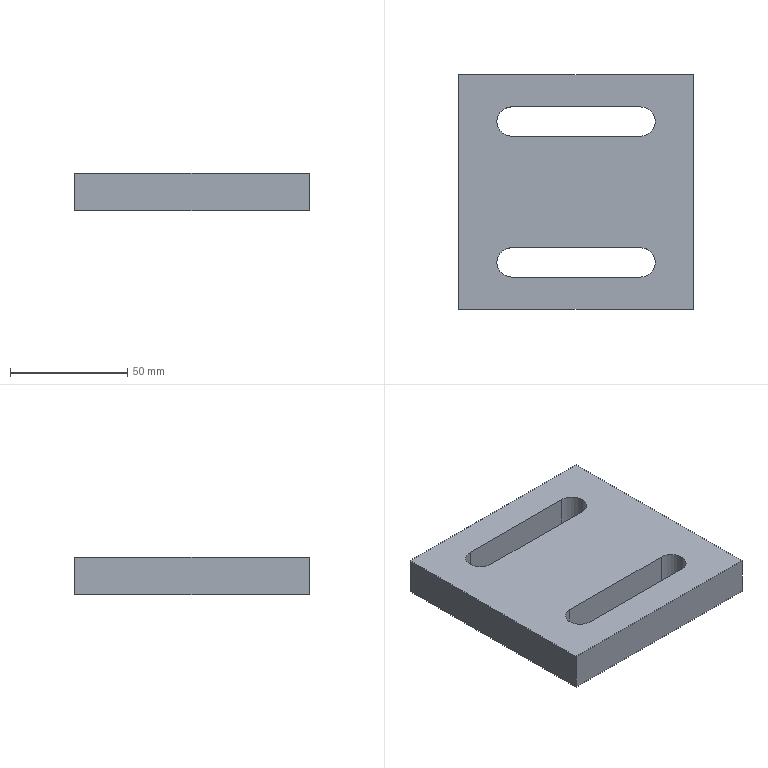Part | STEP file | 1 solid | 16 faces | box 100 x 100 x 16 mm | volume 134073 mm3 | plane 10 | cylinder 6 | commonest cylinder face diameters 12.5 x6
STEP:
#1=CARTESIAN_POINT('',(0.,0.,0.));
#2=DIRECTION('',(0.,0.,1.));
#3=DIRECTION('',(1.,0.,0.));
#4=AXIS2_PLACEMENT_3D('',#1,#2,#3);
#5=CARTESIAN_POINT('',(-27.5,36.25,16.));
#6=VERTEX_POINT('',#5);
#7=CARTESIAN_POINT('',(-27.5,36.25,0.));
#8=VERTEX_POINT('',#7);
#9=CARTESIAN_POINT('',(-27.5,36.25,16.));
#10=DIRECTION('',(0.,0.,-1.));
#11=VECTOR('',#10,1.);
#12=LINE('',#9,#11);
#13=CARTESIAN_POINT('',(-27.5,30.,16.));
#14=DIRECTION('',(0.,0.,-1.));
#15=DIRECTION('',(-1.,0.,0.));
#16=AXIS2_PLACEMENT_3D('',#13,#14,#15);
#17=CYLINDRICAL_SURFACE('',#16,6.25);
#18=CARTESIAN_POINT('',(1.571,0.));
#19=DIRECTION('',(0.,1.));
#20=VECTOR('',#19,1.);
#21=LINE('',#18,#20);
#22=(GEOMETRIC_REPRESENTATION_CONTEXT(2)PARAMETRIC_REPRESENTATION_CONTEXT()REPRESENTATION_CONTEXT('',''));
#23=DEFINITIONAL_REPRESENTATION('',(#21),#22);
#24=PCURVE('',#17,#23);
#25=CARTESIAN_POINT('',(-27.5,36.25,16.));
#26=DIRECTION('',(0.,-1.,0.));
#27=DIRECTION('',(0.,0.,-1.));
#28=AXIS2_PLACEMENT_3D('',#25,#26,#27);
#29=PLANE('',#28);
#30=CARTESIAN_POINT('',(0.,0.));
#31=DIRECTION('',(1.,0.));
#32=VECTOR('',#31,1.);
#33=LINE('',#30,#32);
#34=(GEOMETRIC_REPRESENTATION_CONTEXT(2)PARAMETRIC_REPRESENTATION_CONTEXT()REPRESENTATION_CONTEXT('',''));
#35=DEFINITIONAL_REPRESENTATION('',(#33),#34);
#36=PCURVE('',#29,#35);
#37=SURFACE_CURVE('',#12,(#24,#36),.PCURVE_S1.);
#38=EDGE_CURVE('',#6,#8,#37,.T.);
#39=ORIENTED_EDGE('',*,*,#38,.T.);
#40=CARTESIAN_POINT('',(-33.75,30.,0.));
#41=VERTEX_POINT('',#40);
#42=CARTESIAN_POINT('',(-27.5,30.,0.));
#43=DIRECTION('',(0.,0.,1.));
#44=DIRECTION('',(1.,0.,0.));
#45=AXIS2_PLACEMENT_3D('',#42,#43,#44);
#46=CIRCLE('',#45,6.25);
#47=CARTESIAN_POINT('',(3.142,16.));
#48=DIRECTION('',(-1.,0.));
#49=VECTOR('',#48,1.);
#50=LINE('',#47,#49);
#51=(GEOMETRIC_REPRESENTATION_CONTEXT(2)PARAMETRIC_REPRESENTATION_CONTEXT()REPRESENTATION_CONTEXT('',''));
#52=DEFINITIONAL_REPRESENTATION('',(#50),#51);
#53=PCURVE('',#17,#52);
#54=CARTESIAN_POINT('',(0.,0.,0.));
#55=DIRECTION('',(0.,0.,1.));
#56=DIRECTION('',(1.,0.,0.));
#57=AXIS2_PLACEMENT_3D('',#54,#55,#56);
#58=PLANE('',#57);
#59=CARTESIAN_POINT('',(-27.5,30.));
#60=DIRECTION('',(1.,0.));
#61=AXIS2_PLACEMENT_2D('',#59,#60);
#62=CIRCLE('',#61,6.25);
#63=(GEOMETRIC_REPRESENTATION_CONTEXT(2)PARAMETRIC_REPRESENTATION_CONTEXT()REPRESENTATION_CONTEXT('',''));
#64=DEFINITIONAL_REPRESENTATION('',(#62),#63);
#65=PCURVE('',#58,#64);
#66=SURFACE_CURVE('',#46,(#53,#65),.PCURVE_S1.);
#67=EDGE_CURVE('',#8,#41,#66,.T.);
#68=ORIENTED_EDGE('',*,*,#67,.T.);
#69=CARTESIAN_POINT('',(-33.75,30.,16.));
#70=VERTEX_POINT('',#69);
#71=CARTESIAN_POINT('',(-33.75,30.,16.));
#72=DIRECTION('',(0.,0.,-1.));
#73=VECTOR('',#72,1.);
#74=LINE('',#71,#73);
#75=CARTESIAN_POINT('',(0.,0.));
#76=DIRECTION('',(0.,1.));
#77=VECTOR('',#76,1.);
#78=LINE('',#75,#77);
#79=(GEOMETRIC_REPRESENTATION_CONTEXT(2)PARAMETRIC_REPRESENTATION_CONTEXT()REPRESENTATION_CONTEXT('',''));
#80=DEFINITIONAL_REPRESENTATION('',(#78),#79);
#81=PCURVE('',#17,#80);
#82=CARTESIAN_POINT('',(-27.5,30.,16.));
#83=DIRECTION('',(0.,0.,-1.));
#84=DIRECTION('',(-1.,0.,0.));
#85=AXIS2_PLACEMENT_3D('',#82,#83,#84);
#86=CYLINDRICAL_SURFACE('',#85,6.25);
#87=CARTESIAN_POINT('',(6.283,0.));
#88=DIRECTION('',(0.,1.));
#89=VECTOR('',#88,1.);
#90=LINE('',#87,#89);
#91=(GEOMETRIC_REPRESENTATION_CONTEXT(2)PARAMETRIC_REPRESENTATION_CONTEXT()REPRESENTATION_CONTEXT('',''));
#92=DEFINITIONAL_REPRESENTATION('',(#90),#91);
#93=PCURVE('',#86,#92);
#94=SURFACE_CURVE('',#74,(#81,#93),.PCURVE_S1.);
#95=EDGE_CURVE('',#70,#41,#94,.T.);
#96=ORIENTED_EDGE('',*,*,#95,.F.);
#97=CARTESIAN_POINT('',(-27.5,30.,16.));
#98=DIRECTION('',(0.,0.,1.));
#99=DIRECTION('',(1.,0.,0.));
#100=AXIS2_PLACEMENT_3D('',#97,#98,#99);
#101=CIRCLE('',#100,6.25);
#102=CARTESIAN_POINT('',(3.142,0.));
#103=DIRECTION('',(-1.,0.));
#104=VECTOR('',#103,1.);
#105=LINE('',#102,#104);
#106=(GEOMETRIC_REPRESENTATION_CONTEXT(2)PARAMETRIC_REPRESENTATION_CONTEXT()REPRESENTATION_CONTEXT('',''));
#107=DEFINITIONAL_REPRESENTATION('',(#105),#106);
#108=PCURVE('',#17,#107);
#109=CARTESIAN_POINT('',(0.,0.,16.));
#110=DIRECTION('',(0.,0.,1.));
#111=DIRECTION('',(1.,0.,0.));
#112=AXIS2_PLACEMENT_3D('',#109,#110,#111);
#113=PLANE('',#112);
#114=CARTESIAN_POINT('',(-27.5,30.));
#115=DIRECTION('',(1.,0.));
#116=AXIS2_PLACEMENT_2D('',#114,#115);
#117=CIRCLE('',#116,6.25);
#118=(GEOMETRIC_REPRESENTATION_CONTEXT(2)PARAMETRIC_REPRESENTATION_CONTEXT()REPRESENTATION_CONTEXT('',''));
#119=DEFINITIONAL_REPRESENTATION('',(#117),#118);
#120=PCURVE('',#113,#119);
#121=SURFACE_CURVE('',#101,(#108,#120),.PCURVE_S1.);
#122=EDGE_CURVE('',#6,#70,#121,.T.);
#123=ORIENTED_EDGE('',*,*,#122,.F.);
#124=EDGE_LOOP('',(#39,#68,#96,#123));
#125=FACE_BOUND('',#124,.F.);
#126=ADVANCED_FACE('',(#125),#17,.F.);
#127=CARTESIAN_POINT('',(-27.5,-23.75,16.));
#128=VERTEX_POINT('',#127);
#129=CARTESIAN_POINT('',(-27.5,-23.75,0.));
#130=VERTEX_POINT('',#129);
#131=CARTESIAN_POINT('',(-27.5,-23.75,16.));
#132=DIRECTION('',(0.,0.,-1.));
#133=VECTOR('',#132,1.);
#134=LINE('',#131,#133);
#135=CARTESIAN_POINT('',(-27.5,-30.,16.));
#136=DIRECTION('',(0.,0.,-1.));
#137=DIRECTION('',(-1.,0.,0.));
#138=AXIS2_PLACEMENT_3D('',#135,#136,#137);
#139=CYLINDRICAL_SURFACE('',#138,6.25);
#140=CARTESIAN_POINT('',(1.571,0.));
#141=DIRECTION('',(0.,1.));
#142=VECTOR('',#141,1.);
#143=LINE('',#140,#142);
#144=(GEOMETRIC_REPRESENTATION_CONTEXT(2)PARAMETRIC_REPRESENTATION_CONTEXT()REPRESENTATION_CONTEXT('',''));
#145=DEFINITIONAL_REPRESENTATION('',(#143),#144);
#146=PCURVE('',#139,#145);
#147=CARTESIAN_POINT('',(-27.5,-23.75,16.));
#148=DIRECTION('',(0.,-1.,0.));
#149=DIRECTION('',(1.,0.,0.));
#150=AXIS2_PLACEMENT_3D('',#147,#148,#149);
#151=PLANE('',#150);
#152=CARTESIAN_POINT('',(0.,0.));
#153=DIRECTION('',(0.,-1.));
#154=VECTOR('',#153,1.);
#155=LINE('',#152,#154);
#156=(GEOMETRIC_REPRESENTATION_CONTEXT(2)PARAMETRIC_REPRESENTATION_CONTEXT()REPRESENTATION_CONTEXT('',''));
#157=DEFINITIONAL_REPRESENTATION('',(#155),#156);
#158=PCURVE('',#151,#157);
#159=SURFACE_CURVE('',#134,(#146,#158),.PCURVE_S1.);
#160=EDGE_CURVE('',#128,#130,#159,.T.);
#161=ORIENTED_EDGE('',*,*,#160,.T.);
#162=CARTESIAN_POINT('',(-33.75,-30.,0.));
#163=VERTEX_POINT('',#162);
#164=CARTESIAN_POINT('',(-27.5,-30.,0.));
#165=DIRECTION('',(0.,0.,1.));
#166=DIRECTION('',(1.,0.,0.));
#167=AXIS2_PLACEMENT_3D('',#164,#165,#166);
#168=CIRCLE('',#167,6.25);
#169=CARTESIAN_POINT('',(3.142,16.));
#170=DIRECTION('',(-1.,0.));
#171=VECTOR('',#170,1.);
#172=LINE('',#169,#171);
#173=(GEOMETRIC_REPRESENTATION_CONTEXT(2)PARAMETRIC_REPRESENTATION_CONTEXT()REPRESENTATION_CONTEXT('',''));
#174=DEFINITIONAL_REPRESENTATION('',(#172),#173);
#175=PCURVE('',#139,#174);
#176=CARTESIAN_POINT('',(-27.5,-30.));
#177=DIRECTION('',(1.,0.));
#178=AXIS2_PLACEMENT_2D('',#176,#177);
#179=CIRCLE('',#178,6.25);
#180=(GEOMETRIC_REPRESENTATION_CONTEXT(2)PARAMETRIC_REPRESENTATION_CONTEXT()REPRESENTATION_CONTEXT('',''));
#181=DEFINITIONAL_REPRESENTATION('',(#179),#180);
#182=PCURVE('',#58,#181);
#183=SURFACE_CURVE('',#168,(#175,#182),.PCURVE_S1.);
#184=EDGE_CURVE('',#130,#163,#183,.T.);
#185=ORIENTED_EDGE('',*,*,#184,.T.);
#186=CARTESIAN_POINT('',(-33.75,-30.,16.));
#187=VERTEX_POINT('',#186);
#188=CARTESIAN_POINT('',(-33.75,-30.,16.));
#189=DIRECTION('',(0.,0.,-1.));
#190=VECTOR('',#189,1.);
#191=LINE('',#188,#190);
#192=CARTESIAN_POINT('',(0.,0.));
#193=DIRECTION('',(0.,1.));
#194=VECTOR('',#193,1.);
#195=LINE('',#192,#194);
#196=(GEOMETRIC_REPRESENTATION_CONTEXT(2)PARAMETRIC_REPRESENTATION_CONTEXT()REPRESENTATION_CONTEXT('',''));
#197=DEFINITIONAL_REPRESENTATION('',(#195),#196);
#198=PCURVE('',#139,#197);
#199=CARTESIAN_POINT('',(-27.5,-30.,16.));
#200=DIRECTION('',(0.,0.,-1.));
#201=DIRECTION('',(-1.,0.,0.));
#202=AXIS2_PLACEMENT_3D('',#199,#200,#201);
#203=CYLINDRICAL_SURFACE('',#202,6.25);
#204=CARTESIAN_POINT('',(6.283,0.));
#205=DIRECTION('',(0.,1.));
#206=VECTOR('',#205,1.);
#207=LINE('',#204,#206);
#208=(GEOMETRIC_REPRESENTATION_CONTEXT(2)PARAMETRIC_REPRESENTATION_CONTEXT()REPRESENTATION_CONTEXT('',''));
#209=DEFINITIONAL_REPRESENTATION('',(#207),#208);
#210=PCURVE('',#203,#209);
#211=SURFACE_CURVE('',#191,(#198,#210),.PCURVE_S1.);
#212=EDGE_CURVE('',#187,#163,#211,.T.);
#213=ORIENTED_EDGE('',*,*,#212,.F.);
#214=CARTESIAN_POINT('',(-27.5,-30.,16.));
#215=DIRECTION('',(0.,0.,1.));
#216=DIRECTION('',(1.,0.,0.));
#217=AXIS2_PLACEMENT_3D('',#214,#215,#216);
#218=CIRCLE('',#217,6.25);
#219=CARTESIAN_POINT('',(3.142,0.));
#220=DIRECTION('',(-1.,0.));
#221=VECTOR('',#220,1.);
#222=LINE('',#219,#221);
#223=(GEOMETRIC_REPRESENTATION_CONTEXT(2)PARAMETRIC_REPRESENTATION_CONTEXT()REPRESENTATION_CONTEXT('',''));
#224=DEFINITIONAL_REPRESENTATION('',(#222),#223);
#225=PCURVE('',#139,#224);
#226=CARTESIAN_POINT('',(-27.5,-30.));
#227=DIRECTION('',(1.,0.));
#228=AXIS2_PLACEMENT_2D('',#226,#227);
#229=CIRCLE('',#228,6.25);
#230=(GEOMETRIC_REPRESENTATION_CONTEXT(2)PARAMETRIC_REPRESENTATION_CONTEXT()REPRESENTATION_CONTEXT('',''));
#231=DEFINITIONAL_REPRESENTATION('',(#229),#230);
#232=PCURVE('',#113,#231);
#233=SURFACE_CURVE('',#218,(#225,#232),.PCURVE_S1.);
#234=EDGE_CURVE('',#128,#187,#233,.T.);
#235=ORIENTED_EDGE('',*,*,#234,.F.);
#236=EDGE_LOOP('',(#161,#185,#213,#235));
#237=FACE_BOUND('',#236,.F.);
#238=ADVANCED_FACE('',(#237),#139,.F.);
#239=CARTESIAN_POINT('',(50.,-50.,16.));
#240=VERTEX_POINT('',#239);
#241=CARTESIAN_POINT('',(50.,50.,16.));
#242=VERTEX_POINT('',#241);
#243=CARTESIAN_POINT('',(50.,-10.,16.));
#244=DIRECTION('',(0.,1.,0.));
#245=VECTOR('',#244,1.);
#246=LINE('',#243,#245);
#247=CARTESIAN_POINT('',(50.,-10.));
#248=DIRECTION('',(0.,1.));
#249=VECTOR('',#248,1.);
#250=LINE('',#247,#249);
#251=(GEOMETRIC_REPRESENTATION_CONTEXT(2)PARAMETRIC_REPRESENTATION_CONTEXT()REPRESENTATION_CONTEXT('',''));
#252=DEFINITIONAL_REPRESENTATION('',(#250),#251);
#253=PCURVE('',#113,#252);
#254=CARTESIAN_POINT('',(50.,50.,16.));
#255=DIRECTION('',(-1.,0.,0.));
#256=DIRECTION('',(0.,-1.,0.));
#257=AXIS2_PLACEMENT_3D('',#254,#255,#256);
#258=PLANE('',#257);
#259=CARTESIAN_POINT('',(60.,0.));
#260=DIRECTION('',(-1.,0.));
#261=VECTOR('',#260,1.);
#262=LINE('',#259,#261);
#263=(GEOMETRIC_REPRESENTATION_CONTEXT(2)PARAMETRIC_REPRESENTATION_CONTEXT()REPRESENTATION_CONTEXT('',''));
#264=DEFINITIONAL_REPRESENTATION('',(#262),#263);
#265=PCURVE('',#258,#264);
#266=SURFACE_CURVE('',#246,(#253,#265),.PCURVE_S1.);
#267=EDGE_CURVE('',#240,#242,#266,.T.);
#268=ORIENTED_EDGE('',*,*,#267,.T.);
#269=CARTESIAN_POINT('',(-50.,50.,16.));
#270=VERTEX_POINT('',#269);
#271=CARTESIAN_POINT('',(-50.,50.,16.));
#272=DIRECTION('',(-1.,0.,0.));
#273=VECTOR('',#272,1.);
#274=LINE('',#271,#273);
#275=CARTESIAN_POINT('',(-50.,50.));
#276=DIRECTION('',(-1.,0.));
#277=VECTOR('',#276,1.);
#278=LINE('',#275,#277);
#279=(GEOMETRIC_REPRESENTATION_CONTEXT(2)PARAMETRIC_REPRESENTATION_CONTEXT()REPRESENTATION_CONTEXT('',''));
#280=DEFINITIONAL_REPRESENTATION('',(#278),#279);
#281=PCURVE('',#113,#280);
#282=CARTESIAN_POINT('',(-50.,50.,16.));
#283=DIRECTION('',(0.,-1.,0.));
#284=DIRECTION('',(0.,0.,-1.));
#285=AXIS2_PLACEMENT_3D('',#282,#283,#284);
#286=PLANE('',#285);
#287=CARTESIAN_POINT('',(0.,0.));
#288=DIRECTION('',(0.,-1.));
#289=VECTOR('',#288,1.);
#290=LINE('',#287,#289);
#291=(GEOMETRIC_REPRESENTATION_CONTEXT(2)PARAMETRIC_REPRESENTATION_CONTEXT()REPRESENTATION_CONTEXT('',''));
#292=DEFINITIONAL_REPRESENTATION('',(#290),#291);
#293=PCURVE('',#286,#292);
#294=SURFACE_CURVE('',#274,(#281,#293),.PCURVE_S1.);
#295=EDGE_CURVE('',#242,#270,#294,.T.);
#296=ORIENTED_EDGE('',*,*,#295,.T.);
#297=CARTESIAN_POINT('',(-50.,-50.,16.));
#298=VERTEX_POINT('',#297);
#299=CARTESIAN_POINT('',(-50.,50.,16.));
#300=DIRECTION('',(0.,-1.,0.));
#301=VECTOR('',#300,1.);
#302=LINE('',#299,#301);
#303=CARTESIAN_POINT('',(-50.,50.));
#304=DIRECTION('',(0.,-1.));
#305=VECTOR('',#304,1.);
#306=LINE('',#303,#305);
#307=(GEOMETRIC_REPRESENTATION_CONTEXT(2)PARAMETRIC_REPRESENTATION_CONTEXT()REPRESENTATION_CONTEXT('',''));
#308=DEFINITIONAL_REPRESENTATION('',(#306),#307);
#309=PCURVE('',#113,#308);
#310=CARTESIAN_POINT('',(-50.,50.,16.));
#311=DIRECTION('',(1.,0.,0.));
#312=DIRECTION('',(0.,1.,0.));
#313=AXIS2_PLACEMENT_3D('',#310,#311,#312);
#314=PLANE('',#313);
#315=CARTESIAN_POINT('',(0.,0.));
#316=DIRECTION('',(-1.,0.));
#317=VECTOR('',#316,1.);
#318=LINE('',#315,#317);
#319=(GEOMETRIC_REPRESENTATION_CONTEXT(2)PARAMETRIC_REPRESENTATION_CONTEXT()REPRESENTATION_CONTEXT('',''));
#320=DEFINITIONAL_REPRESENTATION('',(#318),#319);
#321=PCURVE('',#314,#320);
#322=SURFACE_CURVE('',#302,(#309,#321),.PCURVE_S1.);
#323=EDGE_CURVE('',#270,#298,#322,.T.);
#324=ORIENTED_EDGE('',*,*,#323,.T.);
#325=CARTESIAN_POINT('',(-50.,-50.,16.));
#326=DIRECTION('',(1.,0.,0.));
#327=VECTOR('',#326,1.);
#328=LINE('',#325,#327);
#329=CARTESIAN_POINT('',(-50.,-50.));
#330=DIRECTION('',(1.,0.));
#331=VECTOR('',#330,1.);
#332=LINE('',#329,#331);
#333=(GEOMETRIC_REPRESENTATION_CONTEXT(2)PARAMETRIC_REPRESENTATION_CONTEXT()REPRESENTATION_CONTEXT('',''));
#334=DEFINITIONAL_REPRESENTATION('',(#332),#333);
#335=PCURVE('',#113,#334);
#336=CARTESIAN_POINT('',(-50.,-50.,16.));
#337=DIRECTION('',(0.,1.,0.));
#338=DIRECTION('',(0.,0.,1.));
#339=AXIS2_PLACEMENT_3D('',#336,#337,#338);
#340=PLANE('',#339);
#341=CARTESIAN_POINT('',(0.,0.));
#342=DIRECTION('',(0.,1.));
#343=VECTOR('',#342,1.);
#344=LINE('',#341,#343);
#345=(GEOMETRIC_REPRESENTATION_CONTEXT(2)PARAMETRIC_REPRESENTATION_CONTEXT()REPRESENTATION_CONTEXT('',''));
#346=DEFINITIONAL_REPRESENTATION('',(#344),#345);
#347=PCURVE('',#340,#346);
#348=SURFACE_CURVE('',#328,(#335,#347),.PCURVE_S1.);
#349=EDGE_CURVE('',#298,#240,#348,.T.);
#350=ORIENTED_EDGE('',*,*,#349,.T.);
#351=EDGE_LOOP('',(#268,#296,#324,#350));
#352=FACE_BOUND('',#351,.T.);
#353=CARTESIAN_POINT('',(-27.5,-36.25,16.));
#354=VERTEX_POINT('',#353);
#355=CARTESIAN_POINT('',(27.5,-36.25,16.));
#356=VERTEX_POINT('',#355);
#357=CARTESIAN_POINT('',(-27.5,-36.25,16.));
#358=DIRECTION('',(1.,0.,0.));
#359=VECTOR('',#358,1.);
#360=LINE('',#357,#359);
#361=CARTESIAN_POINT('',(-27.5,-36.25));
#362=DIRECTION('',(1.,0.));
#363=VECTOR('',#362,1.);
#364=LINE('',#361,#363);
#365=(GEOMETRIC_REPRESENTATION_CONTEXT(2)PARAMETRIC_REPRESENTATION_CONTEXT()REPRESENTATION_CONTEXT('',''));
#366=DEFINITIONAL_REPRESENTATION('',(#364),#365);
#367=PCURVE('',#113,#366);
#368=CARTESIAN_POINT('',(-27.5,-36.25,16.));
#369=DIRECTION('',(0.,1.,0.));
#370=DIRECTION('',(0.,0.,1.));
#371=AXIS2_PLACEMENT_3D('',#368,#369,#370);
#372=PLANE('',#371);
#373=CARTESIAN_POINT('',(0.,0.));
#374=DIRECTION('',(0.,1.));
#375=VECTOR('',#374,1.);
#376=LINE('',#373,#375);
#377=(GEOMETRIC_REPRESENTATION_CONTEXT(2)PARAMETRIC_REPRESENTATION_CONTEXT()REPRESENTATION_CONTEXT('',''));
#378=DEFINITIONAL_REPRESENTATION('',(#376),#377);
#379=PCURVE('',#372,#378);
#380=SURFACE_CURVE('',#360,(#367,#379),.PCURVE_S1.);
#381=EDGE_CURVE('',#354,#356,#380,.T.);
#382=ORIENTED_EDGE('',*,*,#381,.F.);
#383=CARTESIAN_POINT('',(-27.5,-30.,16.));
#384=DIRECTION('',(0.,0.,1.));
#385=DIRECTION('',(1.,0.,0.));
#386=AXIS2_PLACEMENT_3D('',#383,#384,#385);
#387=CIRCLE('',#386,6.25);
#388=CARTESIAN_POINT('',(-27.5,-30.));
#389=DIRECTION('',(1.,0.));
#390=AXIS2_PLACEMENT_2D('',#388,#389);
#391=CIRCLE('',#390,6.25);
#392=(GEOMETRIC_REPRESENTATION_CONTEXT(2)PARAMETRIC_REPRESENTATION_CONTEXT()REPRESENTATION_CONTEXT('',''));
#393=DEFINITIONAL_REPRESENTATION('',(#391),#392);
#394=PCURVE('',#113,#393);
#395=CARTESIAN_POINT('',(9.425,0.));
#396=DIRECTION('',(-1.,0.));
#397=VECTOR('',#396,1.);
#398=LINE('',#395,#397);
#399=(GEOMETRIC_REPRESENTATION_CONTEXT(2)PARAMETRIC_REPRESENTATION_CONTEXT()REPRESENTATION_CONTEXT('',''));
#400=DEFINITIONAL_REPRESENTATION('',(#398),#399);
#401=PCURVE('',#203,#400);
#402=SURFACE_CURVE('',#387,(#394,#401),.PCURVE_S1.);
#403=EDGE_CURVE('',#187,#354,#402,.T.);
#404=ORIENTED_EDGE('',*,*,#403,.F.);
#405=ORIENTED_EDGE('',*,*,#234,.F.);
#406=CARTESIAN_POINT('',(27.5,-23.75,16.));
#407=VERTEX_POINT('',#406);
#408=CARTESIAN_POINT('',(-27.5,-23.75,16.));
#409=DIRECTION('',(-1.,0.,0.));
#410=VECTOR('',#409,1.);
#411=LINE('',#408,#410);
#412=CARTESIAN_POINT('',(-27.5,-23.75));
#413=DIRECTION('',(-1.,0.));
#414=VECTOR('',#413,1.);
#415=LINE('',#412,#414);
#416=(GEOMETRIC_REPRESENTATION_CONTEXT(2)PARAMETRIC_REPRESENTATION_CONTEXT()REPRESENTATION_CONTEXT('',''));
#417=DEFINITIONAL_REPRESENTATION('',(#415),#416);
#418=PCURVE('',#113,#417);
#419=CARTESIAN_POINT('',(0.,0.));
#420=DIRECTION('',(-1.,0.));
#421=VECTOR('',#420,1.);
#422=LINE('',#419,#421);
#423=(GEOMETRIC_REPRESENTATION_CONTEXT(2)PARAMETRIC_REPRESENTATION_CONTEXT()REPRESENTATION_CONTEXT('',''));
#424=DEFINITIONAL_REPRESENTATION('',(#422),#423);
#425=PCURVE('',#151,#424);
#426=SURFACE_CURVE('',#411,(#418,#425),.PCURVE_S1.);
#427=EDGE_CURVE('',#407,#128,#426,.T.);
#428=ORIENTED_EDGE('',*,*,#427,.F.);
#429=CARTESIAN_POINT('',(27.5,-30.,16.));
#430=DIRECTION('',(0.,0.,1.));
#431=DIRECTION('',(1.,0.,0.));
#432=AXIS2_PLACEMENT_3D('',#429,#430,#431);
#433=CIRCLE('',#432,6.25);
#434=CARTESIAN_POINT('',(27.5,-30.));
#435=DIRECTION('',(1.,0.));
#436=AXIS2_PLACEMENT_2D('',#434,#435);
#437=CIRCLE('',#436,6.25);
#438=(GEOMETRIC_REPRESENTATION_CONTEXT(2)PARAMETRIC_REPRESENTATION_CONTEXT()REPRESENTATION_CONTEXT('',''));
#439=DEFINITIONAL_REPRESENTATION('',(#437),#438);
#440=PCURVE('',#113,#439);
#441=CARTESIAN_POINT('',(27.5,-30.,16.));
#442=DIRECTION('',(0.,0.,-1.));
#443=DIRECTION('',(-1.,0.,0.));
#444=AXIS2_PLACEMENT_3D('',#441,#442,#443);
#445=CYLINDRICAL_SURFACE('',#444,6.25);
#446=CARTESIAN_POINT('',(9.425,0.));
#447=DIRECTION('',(-1.,0.));
#448=VECTOR('',#447,1.);
#449=LINE('',#446,#448);
#450=(GEOMETRIC_REPRESENTATION_CONTEXT(2)PARAMETRIC_REPRESENTATION_CONTEXT()REPRESENTATION_CONTEXT('',''));
#451=DEFINITIONAL_REPRESENTATION('',(#449),#450);
#452=PCURVE('',#445,#451);
#453=SURFACE_CURVE('',#433,(#440,#452),.PCURVE_S1.);
#454=EDGE_CURVE('',#356,#407,#453,.T.);
#455=ORIENTED_EDGE('',*,*,#454,.F.);
#456=EDGE_LOOP('',(#382,#404,#405,#428,#455));
#457=FACE_BOUND('',#456,.T.);
#458=CARTESIAN_POINT('',(-27.5,23.75,16.));
#459=VERTEX_POINT('',#458);
#460=CARTESIAN_POINT('',(27.5,23.75,16.));
#461=VERTEX_POINT('',#460);
#462=CARTESIAN_POINT('',(-27.5,23.75,16.));
#463=DIRECTION('',(1.,0.,0.));
#464=VECTOR('',#463,1.);
#465=LINE('',#462,#464);
#466=CARTESIAN_POINT('',(-27.5,23.75));
#467=DIRECTION('',(1.,0.));
#468=VECTOR('',#467,1.);
#469=LINE('',#466,#468);
#470=(GEOMETRIC_REPRESENTATION_CONTEXT(2)PARAMETRIC_REPRESENTATION_CONTEXT()REPRESENTATION_CONTEXT('',''));
#471=DEFINITIONAL_REPRESENTATION('',(#469),#470);
#472=PCURVE('',#113,#471);
#473=CARTESIAN_POINT('',(-27.5,23.75,16.));
#474=DIRECTION('',(0.,1.,0.));
#475=DIRECTION('',(0.,0.,1.));
#476=AXIS2_PLACEMENT_3D('',#473,#474,#475);
#477=PLANE('',#476);
#478=CARTESIAN_POINT('',(0.,0.));
#479=DIRECTION('',(0.,1.));
#480=VECTOR('',#479,1.);
#481=LINE('',#478,#480);
#482=(GEOMETRIC_REPRESENTATION_CONTEXT(2)PARAMETRIC_REPRESENTATION_CONTEXT()REPRESENTATION_CONTEXT('',''));
#483=DEFINITIONAL_REPRESENTATION('',(#481),#482);
#484=PCURVE('',#477,#483);
#485=SURFACE_CURVE('',#465,(#472,#484),.PCURVE_S1.);
#486=EDGE_CURVE('',#459,#461,#485,.T.);
#487=ORIENTED_EDGE('',*,*,#486,.F.);
#488=CARTESIAN_POINT('',(-27.5,30.,16.));
#489=DIRECTION('',(0.,0.,1.));
#490=DIRECTION('',(1.,0.,0.));
#491=AXIS2_PLACEMENT_3D('',#488,#489,#490);
#492=CIRCLE('',#491,6.25);
#493=CARTESIAN_POINT('',(-27.5,30.));
#494=DIRECTION('',(1.,0.));
#495=AXIS2_PLACEMENT_2D('',#493,#494);
#496=CIRCLE('',#495,6.25);
#497=(GEOMETRIC_REPRESENTATION_CONTEXT(2)PARAMETRIC_REPRESENTATION_CONTEXT()REPRESENTATION_CONTEXT('',''));
#498=DEFINITIONAL_REPRESENTATION('',(#496),#497);
#499=PCURVE('',#113,#498);
#500=CARTESIAN_POINT('',(9.425,0.));
#501=DIRECTION('',(-1.,0.));
#502=VECTOR('',#501,1.);
#503=LINE('',#500,#502);
#504=(GEOMETRIC_REPRESENTATION_CONTEXT(2)PARAMETRIC_REPRESENTATION_CONTEXT()REPRESENTATION_CONTEXT('',''));
#505=DEFINITIONAL_REPRESENTATION('',(#503),#504);
#506=PCURVE('',#86,#505);
#507=SURFACE_CURVE('',#492,(#499,#506),.PCURVE_S1.);
#508=EDGE_CURVE('',#70,#459,#507,.T.);
#509=ORIENTED_EDGE('',*,*,#508,.F.);
#510=ORIENTED_EDGE('',*,*,#122,.F.);
#511=CARTESIAN_POINT('',(27.5,36.25,16.));
#512=VERTEX_POINT('',#511);
#513=CARTESIAN_POINT('',(-27.5,36.25,16.));
#514=DIRECTION('',(-1.,0.,0.));
#515=VECTOR('',#514,1.);
#516=LINE('',#513,#515);
#517=CARTESIAN_POINT('',(-27.5,36.25));
#518=DIRECTION('',(-1.,0.));
#519=VECTOR('',#518,1.);
#520=LINE('',#517,#519);
#521=(GEOMETRIC_REPRESENTATION_CONTEXT(2)PARAMETRIC_REPRESENTATION_CONTEXT()REPRESENTATION_CONTEXT('',''));
#522=DEFINITIONAL_REPRESENTATION('',(#520),#521);
#523=PCURVE('',#113,#522);
#524=CARTESIAN_POINT('',(0.,0.));
#525=DIRECTION('',(0.,-1.));
#526=VECTOR('',#525,1.);
#527=LINE('',#524,#526);
#528=(GEOMETRIC_REPRESENTATION_CONTEXT(2)PARAMETRIC_REPRESENTATION_CONTEXT()REPRESENTATION_CONTEXT('',''));
#529=DEFINITIONAL_REPRESENTATION('',(#527),#528);
#530=PCURVE('',#29,#529);
#531=SURFACE_CURVE('',#516,(#523,#530),.PCURVE_S1.);
#532=EDGE_CURVE('',#512,#6,#531,.T.);
#533=ORIENTED_EDGE('',*,*,#532,.F.);
#534=CARTESIAN_POINT('',(27.5,30.,16.));
#535=DIRECTION('',(0.,0.,1.));
#536=DIRECTION('',(1.,0.,0.));
#537=AXIS2_PLACEMENT_3D('',#534,#535,#536);
#538=CIRCLE('',#537,6.25);
#539=CARTESIAN_POINT('',(27.5,30.));
#540=DIRECTION('',(1.,0.));
#541=AXIS2_PLACEMENT_2D('',#539,#540);
#542=CIRCLE('',#541,6.25);
#543=(GEOMETRIC_REPRESENTATION_CONTEXT(2)PARAMETRIC_REPRESENTATION_CONTEXT()REPRESENTATION_CONTEXT('',''));
#544=DEFINITIONAL_REPRESENTATION('',(#542),#543);
#545=PCURVE('',#113,#544);
#546=CARTESIAN_POINT('',(27.5,30.,16.));
#547=DIRECTION('',(0.,0.,-1.));
#548=DIRECTION('',(-1.,0.,0.));
#549=AXIS2_PLACEMENT_3D('',#546,#547,#548);
#550=CYLINDRICAL_SURFACE('',#549,6.25);
#551=CARTESIAN_POINT('',(9.425,0.));
#552=DIRECTION('',(-1.,0.));
#553=VECTOR('',#552,1.);
#554=LINE('',#551,#553);
#555=(GEOMETRIC_REPRESENTATION_CONTEXT(2)PARAMETRIC_REPRESENTATION_CONTEXT()REPRESENTATION_CONTEXT('',''));
#556=DEFINITIONAL_REPRESENTATION('',(#554),#555);
#557=PCURVE('',#550,#556);
#558=SURFACE_CURVE('',#538,(#545,#557),.PCURVE_S1.);
#559=EDGE_CURVE('',#461,#512,#558,.T.);
#560=ORIENTED_EDGE('',*,*,#559,.F.);
#561=EDGE_LOOP('',(#487,#509,#510,#533,#560));
#562=FACE_BOUND('',#561,.T.);
#563=ADVANCED_FACE('',(#352,#457,#562),#113,.T.);
#564=ORIENTED_EDGE('',*,*,#184,.T.);
#565=CARTESIAN_POINT('',(-27.5,-36.25,0.));
#566=VERTEX_POINT('',#565);
#567=CARTESIAN_POINT('',(-27.5,-30.,0.));
#568=DIRECTION('',(0.,0.,1.));
#569=DIRECTION('',(1.,0.,0.));
#570=AXIS2_PLACEMENT_3D('',#567,#568,#569);
#571=CIRCLE('',#570,6.25);
#572=CARTESIAN_POINT('',(-27.5,-30.));
#573=DIRECTION('',(1.,0.));
#574=AXIS2_PLACEMENT_2D('',#572,#573);
#575=CIRCLE('',#574,6.25);
#576=(GEOMETRIC_REPRESENTATION_CONTEXT(2)PARAMETRIC_REPRESENTATION_CONTEXT()REPRESENTATION_CONTEXT('',''));
#577=DEFINITIONAL_REPRESENTATION('',(#575),#576);
#578=PCURVE('',#58,#577);
#579=CARTESIAN_POINT('',(9.425,16.));
#580=DIRECTION('',(-1.,0.));
#581=VECTOR('',#580,1.);
#582=LINE('',#579,#581);
#583=(GEOMETRIC_REPRESENTATION_CONTEXT(2)PARAMETRIC_REPRESENTATION_CONTEXT()REPRESENTATION_CONTEXT('',''));
#584=DEFINITIONAL_REPRESENTATION('',(#582),#583);
#585=PCURVE('',#203,#584);
#586=SURFACE_CURVE('',#571,(#578,#585),.PCURVE_S1.);
#587=EDGE_CURVE('',#163,#566,#586,.T.);
#588=ORIENTED_EDGE('',*,*,#587,.T.);
#589=CARTESIAN_POINT('',(27.5,-36.25,0.));
#590=VERTEX_POINT('',#589);
#591=CARTESIAN_POINT('',(-27.5,-36.25,0.));
#592=DIRECTION('',(1.,0.,0.));
#593=VECTOR('',#592,1.);
#594=LINE('',#591,#593);
#595=CARTESIAN_POINT('',(-27.5,-36.25));
#596=DIRECTION('',(1.,0.));
#597=VECTOR('',#596,1.);
#598=LINE('',#595,#597);
#599=(GEOMETRIC_REPRESENTATION_CONTEXT(2)PARAMETRIC_REPRESENTATION_CONTEXT()REPRESENTATION_CONTEXT('',''));
#600=DEFINITIONAL_REPRESENTATION('',(#598),#599);
#601=PCURVE('',#58,#600);
#602=CARTESIAN_POINT('',(-16.,0.));
#603=DIRECTION('',(0.,1.));
#604=VECTOR('',#603,1.);
#605=LINE('',#602,#604);
#606=(GEOMETRIC_REPRESENTATION_CONTEXT(2)PARAMETRIC_REPRESENTATION_CONTEXT()REPRESENTATION_CONTEXT('',''));
#607=DEFINITIONAL_REPRESENTATION('',(#605),#606);
#608=PCURVE('',#372,#607);
#609=SURFACE_CURVE('',#594,(#601,#608),.PCURVE_S1.);
#610=EDGE_CURVE('',#566,#590,#609,.T.);
#611=ORIENTED_EDGE('',*,*,#610,.T.);
#612=CARTESIAN_POINT('',(27.5,-23.75,0.));
#613=VERTEX_POINT('',#612);
#614=CARTESIAN_POINT('',(27.5,-30.,0.));
#615=DIRECTION('',(0.,0.,1.));
#616=DIRECTION('',(1.,0.,0.));
#617=AXIS2_PLACEMENT_3D('',#614,#615,#616);
#618=CIRCLE('',#617,6.25);
#619=CARTESIAN_POINT('',(27.5,-30.));
#620=DIRECTION('',(1.,0.));
#621=AXIS2_PLACEMENT_2D('',#619,#620);
#622=CIRCLE('',#621,6.25);
#623=(GEOMETRIC_REPRESENTATION_CONTEXT(2)PARAMETRIC_REPRESENTATION_CONTEXT()REPRESENTATION_CONTEXT('',''));
#624=DEFINITIONAL_REPRESENTATION('',(#622),#623);
#625=PCURVE('',#58,#624);
#626=CARTESIAN_POINT('',(9.425,16.));
#627=DIRECTION('',(-1.,0.));
#628=VECTOR('',#627,1.);
#629=LINE('',#626,#628);
#630=(GEOMETRIC_REPRESENTATION_CONTEXT(2)PARAMETRIC_REPRESENTATION_CONTEXT()REPRESENTATION_CONTEXT('',''));
#631=DEFINITIONAL_REPRESENTATION('',(#629),#630);
#632=PCURVE('',#445,#631);
#633=SURFACE_CURVE('',#618,(#625,#632),.PCURVE_S1.);
#634=EDGE_CURVE('',#590,#613,#633,.T.);
#635=ORIENTED_EDGE('',*,*,#634,.T.);
#636=CARTESIAN_POINT('',(-27.5,-23.75,0.));
#637=DIRECTION('',(-1.,0.,0.));
#638=VECTOR('',#637,1.);
#639=LINE('',#636,#638);
#640=CARTESIAN_POINT('',(-27.5,-23.75));
#641=DIRECTION('',(-1.,0.));
#642=VECTOR('',#641,1.);
#643=LINE('',#640,#642);
#644=(GEOMETRIC_REPRESENTATION_CONTEXT(2)PARAMETRIC_REPRESENTATION_CONTEXT()REPRESENTATION_CONTEXT('',''));
#645=DEFINITIONAL_REPRESENTATION('',(#643),#644);
#646=PCURVE('',#58,#645);
#647=CARTESIAN_POINT('',(0.,-16.));
#648=DIRECTION('',(-1.,0.));
#649=VECTOR('',#648,1.);
#650=LINE('',#647,#649);
#651=(GEOMETRIC_REPRESENTATION_CONTEXT(2)PARAMETRIC_REPRESENTATION_CONTEXT()REPRESENTATION_CONTEXT('',''));
#652=DEFINITIONAL_REPRESENTATION('',(#650),#651);
#653=PCURVE('',#151,#652);
#654=SURFACE_CURVE('',#639,(#646,#653),.PCURVE_S1.);
#655=EDGE_CURVE('',#613,#130,#654,.T.);
#656=ORIENTED_EDGE('',*,*,#655,.T.);
#657=EDGE_LOOP('',(#564,#588,#611,#635,#656));
#658=FACE_BOUND('',#657,.T.);
#659=CARTESIAN_POINT('',(50.,-50.,0.));
#660=VERTEX_POINT('',#659);
#661=CARTESIAN_POINT('',(50.,50.,0.));
#662=VERTEX_POINT('',#661);
#663=CARTESIAN_POINT('',(50.,50.,0.));
#664=DIRECTION('',(0.,1.,0.));
#665=VECTOR('',#664,1.);
#666=LINE('',#663,#665);
#667=CARTESIAN_POINT('',(50.,50.));
#668=DIRECTION('',(0.,1.));
#669=VECTOR('',#668,1.);
#670=LINE('',#667,#669);
#671=(GEOMETRIC_REPRESENTATION_CONTEXT(2)PARAMETRIC_REPRESENTATION_CONTEXT()REPRESENTATION_CONTEXT('',''));
#672=DEFINITIONAL_REPRESENTATION('',(#670),#671);
#673=PCURVE('',#58,#672);
#674=CARTESIAN_POINT('',(0.,-16.));
#675=DIRECTION('',(-1.,0.));
#676=VECTOR('',#675,1.);
#677=LINE('',#674,#676);
#678=(GEOMETRIC_REPRESENTATION_CONTEXT(2)PARAMETRIC_REPRESENTATION_CONTEXT()REPRESENTATION_CONTEXT('',''));
#679=DEFINITIONAL_REPRESENTATION('',(#677),#678);
#680=PCURVE('',#258,#679);
#681=SURFACE_CURVE('',#666,(#673,#680),.PCURVE_S1.);
#682=EDGE_CURVE('',#660,#662,#681,.T.);
#683=ORIENTED_EDGE('',*,*,#682,.F.);
#684=CARTESIAN_POINT('',(-50.,-50.,0.));
#685=VERTEX_POINT('',#684);
#686=CARTESIAN_POINT('',(-50.,-50.,0.));
#687=DIRECTION('',(1.,0.,0.));
#688=VECTOR('',#687,1.);
#689=LINE('',#686,#688);
#690=CARTESIAN_POINT('',(-50.,-50.));
#691=DIRECTION('',(1.,0.));
#692=VECTOR('',#691,1.);
#693=LINE('',#690,#692);
#694=(GEOMETRIC_REPRESENTATION_CONTEXT(2)PARAMETRIC_REPRESENTATION_CONTEXT()REPRESENTATION_CONTEXT('',''));
#695=DEFINITIONAL_REPRESENTATION('',(#693),#694);
#696=PCURVE('',#58,#695);
#697=CARTESIAN_POINT('',(-16.,0.));
#698=DIRECTION('',(0.,1.));
#699=VECTOR('',#698,1.);
#700=LINE('',#697,#699);
#701=(GEOMETRIC_REPRESENTATION_CONTEXT(2)PARAMETRIC_REPRESENTATION_CONTEXT()REPRESENTATION_CONTEXT('',''));
#702=DEFINITIONAL_REPRESENTATION('',(#700),#701);
#703=PCURVE('',#340,#702);
#704=SURFACE_CURVE('',#689,(#696,#703),.PCURVE_S1.);
#705=EDGE_CURVE('',#685,#660,#704,.T.);
#706=ORIENTED_EDGE('',*,*,#705,.F.);
#707=CARTESIAN_POINT('',(-50.,50.,0.));
#708=VERTEX_POINT('',#707);
#709=CARTESIAN_POINT('',(-50.,50.,0.));
#710=DIRECTION('',(0.,-1.,0.));
#711=VECTOR('',#710,1.);
#712=LINE('',#709,#711);
#713=CARTESIAN_POINT('',(-50.,50.));
#714=DIRECTION('',(0.,-1.));
#715=VECTOR('',#714,1.);
#716=LINE('',#713,#715);
#717=(GEOMETRIC_REPRESENTATION_CONTEXT(2)PARAMETRIC_REPRESENTATION_CONTEXT()REPRESENTATION_CONTEXT('',''));
#718=DEFINITIONAL_REPRESENTATION('',(#716),#717);
#719=PCURVE('',#58,#718);
#720=CARTESIAN_POINT('',(0.,-16.));
#721=DIRECTION('',(-1.,0.));
#722=VECTOR('',#721,1.);
#723=LINE('',#720,#722);
#724=(GEOMETRIC_REPRESENTATION_CONTEXT(2)PARAMETRIC_REPRESENTATION_CONTEXT()REPRESENTATION_CONTEXT('',''));
#725=DEFINITIONAL_REPRESENTATION('',(#723),#724);
#726=PCURVE('',#314,#725);
#727=SURFACE_CURVE('',#712,(#719,#726),.PCURVE_S1.);
#728=EDGE_CURVE('',#708,#685,#727,.T.);
#729=ORIENTED_EDGE('',*,*,#728,.F.);
#730=CARTESIAN_POINT('',(-50.,50.,0.));
#731=DIRECTION('',(-1.,0.,0.));
#732=VECTOR('',#731,1.);
#733=LINE('',#730,#732);
#734=CARTESIAN_POINT('',(-50.,50.));
#735=DIRECTION('',(-1.,0.));
#736=VECTOR('',#735,1.);
#737=LINE('',#734,#736);
#738=(GEOMETRIC_REPRESENTATION_CONTEXT(2)PARAMETRIC_REPRESENTATION_CONTEXT()REPRESENTATION_CONTEXT('',''));
#739=DEFINITIONAL_REPRESENTATION('',(#737),#738);
#740=PCURVE('',#58,#739);
#741=CARTESIAN_POINT('',(16.,0.));
#742=DIRECTION('',(0.,-1.));
#743=VECTOR('',#742,1.);
#744=LINE('',#741,#743);
#745=(GEOMETRIC_REPRESENTATION_CONTEXT(2)PARAMETRIC_REPRESENTATION_CONTEXT()REPRESENTATION_CONTEXT('',''));
#746=DEFINITIONAL_REPRESENTATION('',(#744),#745);
#747=PCURVE('',#286,#746);
#748=SURFACE_CURVE('',#733,(#740,#747),.PCURVE_S1.);
#749=EDGE_CURVE('',#662,#708,#748,.T.);
#750=ORIENTED_EDGE('',*,*,#749,.F.);
#751=EDGE_LOOP('',(#683,#706,#729,#750));
#752=FACE_BOUND('',#751,.T.);
#753=ORIENTED_EDGE('',*,*,#67,.T.);
#754=CARTESIAN_POINT('',(-27.5,23.75,0.));
#755=VERTEX_POINT('',#754);
#756=CARTESIAN_POINT('',(-27.5,30.,0.));
#757=DIRECTION('',(0.,0.,1.));
#758=DIRECTION('',(1.,0.,0.));
#759=AXIS2_PLACEMENT_3D('',#756,#757,#758);
#760=CIRCLE('',#759,6.25);
#761=CARTESIAN_POINT('',(-27.5,30.));
#762=DIRECTION('',(1.,0.));
#763=AXIS2_PLACEMENT_2D('',#761,#762);
#764=CIRCLE('',#763,6.25);
#765=(GEOMETRIC_REPRESENTATION_CONTEXT(2)PARAMETRIC_REPRESENTATION_CONTEXT()REPRESENTATION_CONTEXT('',''));
#766=DEFINITIONAL_REPRESENTATION('',(#764),#765);
#767=PCURVE('',#58,#766);
#768=CARTESIAN_POINT('',(9.425,16.));
#769=DIRECTION('',(-1.,0.));
#770=VECTOR('',#769,1.);
#771=LINE('',#768,#770);
#772=(GEOMETRIC_REPRESENTATION_CONTEXT(2)PARAMETRIC_REPRESENTATION_CONTEXT()REPRESENTATION_CONTEXT('',''));
#773=DEFINITIONAL_REPRESENTATION('',(#771),#772);
#774=PCURVE('',#86,#773);
#775=SURFACE_CURVE('',#760,(#767,#774),.PCURVE_S1.);
#776=EDGE_CURVE('',#41,#755,#775,.T.);
#777=ORIENTED_EDGE('',*,*,#776,.T.);
#778=CARTESIAN_POINT('',(27.5,23.75,0.));
#779=VERTEX_POINT('',#778);
#780=CARTESIAN_POINT('',(-27.5,23.75,0.));
#781=DIRECTION('',(1.,0.,0.));
#782=VECTOR('',#781,1.);
#783=LINE('',#780,#782);
#784=CARTESIAN_POINT('',(-27.5,23.75));
#785=DIRECTION('',(1.,0.));
#786=VECTOR('',#785,1.);
#787=LINE('',#784,#786);
#788=(GEOMETRIC_REPRESENTATION_CONTEXT(2)PARAMETRIC_REPRESENTATION_CONTEXT()REPRESENTATION_CONTEXT('',''));
#789=DEFINITIONAL_REPRESENTATION('',(#787),#788);
#790=PCURVE('',#58,#789);
#791=CARTESIAN_POINT('',(-16.,0.));
#792=DIRECTION('',(0.,1.));
#793=VECTOR('',#792,1.);
#794=LINE('',#791,#793);
#795=(GEOMETRIC_REPRESENTATION_CONTEXT(2)PARAMETRIC_REPRESENTATION_CONTEXT()REPRESENTATION_CONTEXT('',''));
#796=DEFINITIONAL_REPRESENTATION('',(#794),#795);
#797=PCURVE('',#477,#796);
#798=SURFACE_CURVE('',#783,(#790,#797),.PCURVE_S1.);
#799=EDGE_CURVE('',#755,#779,#798,.T.);
#800=ORIENTED_EDGE('',*,*,#799,.T.);
#801=CARTESIAN_POINT('',(27.5,36.25,0.));
#802=VERTEX_POINT('',#801);
#803=CARTESIAN_POINT('',(27.5,30.,0.));
#804=DIRECTION('',(0.,0.,1.));
#805=DIRECTION('',(1.,0.,0.));
#806=AXIS2_PLACEMENT_3D('',#803,#804,#805);
#807=CIRCLE('',#806,6.25);
#808=CARTESIAN_POINT('',(27.5,30.));
#809=DIRECTION('',(1.,0.));
#810=AXIS2_PLACEMENT_2D('',#808,#809);
#811=CIRCLE('',#810,6.25);
#812=(GEOMETRIC_REPRESENTATION_CONTEXT(2)PARAMETRIC_REPRESENTATION_CONTEXT()REPRESENTATION_CONTEXT('',''));
#813=DEFINITIONAL_REPRESENTATION('',(#811),#812);
#814=PCURVE('',#58,#813);
#815=CARTESIAN_POINT('',(9.425,16.));
#816=DIRECTION('',(-1.,0.));
#817=VECTOR('',#816,1.);
#818=LINE('',#815,#817);
#819=(GEOMETRIC_REPRESENTATION_CONTEXT(2)PARAMETRIC_REPRESENTATION_CONTEXT()REPRESENTATION_CONTEXT('',''));
#820=DEFINITIONAL_REPRESENTATION('',(#818),#819);
#821=PCURVE('',#550,#820);
#822=SURFACE_CURVE('',#807,(#814,#821),.PCURVE_S1.);
#823=EDGE_CURVE('',#779,#802,#822,.T.);
#824=ORIENTED_EDGE('',*,*,#823,.T.);
#825=CARTESIAN_POINT('',(-27.5,36.25,0.));
#826=DIRECTION('',(-1.,0.,0.));
#827=VECTOR('',#826,1.);
#828=LINE('',#825,#827);
#829=CARTESIAN_POINT('',(-27.5,36.25));
#830=DIRECTION('',(-1.,0.));
#831=VECTOR('',#830,1.);
#832=LINE('',#829,#831);
#833=(GEOMETRIC_REPRESENTATION_CONTEXT(2)PARAMETRIC_REPRESENTATION_CONTEXT()REPRESENTATION_CONTEXT('',''));
#834=DEFINITIONAL_REPRESENTATION('',(#832),#833);
#835=PCURVE('',#58,#834);
#836=CARTESIAN_POINT('',(16.,0.));
#837=DIRECTION('',(0.,-1.));
#838=VECTOR('',#837,1.);
#839=LINE('',#836,#838);
#840=(GEOMETRIC_REPRESENTATION_CONTEXT(2)PARAMETRIC_REPRESENTATION_CONTEXT()REPRESENTATION_CONTEXT('',''));
#841=DEFINITIONAL_REPRESENTATION('',(#839),#840);
#842=PCURVE('',#29,#841);
#843=SURFACE_CURVE('',#828,(#835,#842),.PCURVE_S1.);
#844=EDGE_CURVE('',#802,#8,#843,.T.);
#845=ORIENTED_EDGE('',*,*,#844,.T.);
#846=EDGE_LOOP('',(#753,#777,#800,#824,#845));
#847=FACE_BOUND('',#846,.T.);
#848=ADVANCED_FACE('',(#658,#752,#847),#58,.F.);
#849=ORIENTED_EDGE('',*,*,#682,.T.);
#850=CARTESIAN_POINT('',(50.,50.,16.));
#851=DIRECTION('',(0.,0.,-1.));
#852=VECTOR('',#851,1.);
#853=LINE('',#850,#852);
#854=CARTESIAN_POINT('',(0.,0.));
#855=DIRECTION('',(0.,-1.));
#856=VECTOR('',#855,1.);
#857=LINE('',#854,#856);
#858=(GEOMETRIC_REPRESENTATION_CONTEXT(2)PARAMETRIC_REPRESENTATION_CONTEXT()REPRESENTATION_CONTEXT('',''));
#859=DEFINITIONAL_REPRESENTATION('',(#857),#858);
#860=PCURVE('',#258,#859);
#861=CARTESIAN_POINT('',(0.,100.));
#862=DIRECTION('',(1.,0.));
#863=VECTOR('',#862,1.);
#864=LINE('',#861,#863);
#865=(GEOMETRIC_REPRESENTATION_CONTEXT(2)PARAMETRIC_REPRESENTATION_CONTEXT()REPRESENTATION_CONTEXT('',''));
#866=DEFINITIONAL_REPRESENTATION('',(#864),#865);
#867=PCURVE('',#286,#866);
#868=SURFACE_CURVE('',#853,(#860,#867),.PCURVE_S1.);
#869=EDGE_CURVE('',#242,#662,#868,.T.);
#870=ORIENTED_EDGE('',*,*,#869,.F.);
#871=ORIENTED_EDGE('',*,*,#267,.F.);
#872=CARTESIAN_POINT('',(50.,-50.,16.));
#873=DIRECTION('',(0.,0.,-1.));
#874=VECTOR('',#873,1.);
#875=LINE('',#872,#874);
#876=CARTESIAN_POINT('',(100.,0.));
#877=DIRECTION('',(0.,-1.));
#878=VECTOR('',#877,1.);
#879=LINE('',#876,#878);
#880=(GEOMETRIC_REPRESENTATION_CONTEXT(2)PARAMETRIC_REPRESENTATION_CONTEXT()REPRESENTATION_CONTEXT('',''));
#881=DEFINITIONAL_REPRESENTATION('',(#879),#880);
#882=PCURVE('',#258,#881);
#883=CARTESIAN_POINT('',(0.,100.));
#884=DIRECTION('',(-1.,0.));
#885=VECTOR('',#884,1.);
#886=LINE('',#883,#885);
#887=(GEOMETRIC_REPRESENTATION_CONTEXT(2)PARAMETRIC_REPRESENTATION_CONTEXT()REPRESENTATION_CONTEXT('',''));
#888=DEFINITIONAL_REPRESENTATION('',(#886),#887);
#889=PCURVE('',#340,#888);
#890=SURFACE_CURVE('',#875,(#882,#889),.PCURVE_S1.);
#891=EDGE_CURVE('',#240,#660,#890,.T.);
#892=ORIENTED_EDGE('',*,*,#891,.T.);
#893=EDGE_LOOP('',(#849,#870,#871,#892));
#894=FACE_BOUND('',#893,.T.);
#895=ADVANCED_FACE('',(#894),#258,.F.);
#896=ORIENTED_EDGE('',*,*,#749,.T.);
#897=CARTESIAN_POINT('',(-50.,50.,16.));
#898=DIRECTION('',(0.,0.,-1.));
#899=VECTOR('',#898,1.);
#900=LINE('',#897,#899);
#901=CARTESIAN_POINT('',(0.,0.));
#902=DIRECTION('',(1.,0.));
#903=VECTOR('',#902,1.);
#904=LINE('',#901,#903);
#905=(GEOMETRIC_REPRESENTATION_CONTEXT(2)PARAMETRIC_REPRESENTATION_CONTEXT()REPRESENTATION_CONTEXT('',''));
#906=DEFINITIONAL_REPRESENTATION('',(#904),#905);
#907=PCURVE('',#286,#906);
#908=CARTESIAN_POINT('',(0.,0.));
#909=DIRECTION('',(0.,-1.));
#910=VECTOR('',#909,1.);
#911=LINE('',#908,#910);
#912=(GEOMETRIC_REPRESENTATION_CONTEXT(2)PARAMETRIC_REPRESENTATION_CONTEXT()REPRESENTATION_CONTEXT('',''));
#913=DEFINITIONAL_REPRESENTATION('',(#911),#912);
#914=PCURVE('',#314,#913);
#915=SURFACE_CURVE('',#900,(#907,#914),.PCURVE_S1.);
#916=EDGE_CURVE('',#270,#708,#915,.T.);
#917=ORIENTED_EDGE('',*,*,#916,.F.);
#918=ORIENTED_EDGE('',*,*,#295,.F.);
#919=ORIENTED_EDGE('',*,*,#869,.T.);
#920=EDGE_LOOP('',(#896,#917,#918,#919));
#921=FACE_BOUND('',#920,.T.);
#922=ADVANCED_FACE('',(#921),#286,.F.);
#923=ORIENTED_EDGE('',*,*,#728,.T.);
#924=CARTESIAN_POINT('',(-50.,-50.,16.));
#925=DIRECTION('',(0.,0.,-1.));
#926=VECTOR('',#925,1.);
#927=LINE('',#924,#926);
#928=CARTESIAN_POINT('',(-100.,0.));
#929=DIRECTION('',(0.,-1.));
#930=VECTOR('',#929,1.);
#931=LINE('',#928,#930);
#932=(GEOMETRIC_REPRESENTATION_CONTEXT(2)PARAMETRIC_REPRESENTATION_CONTEXT()REPRESENTATION_CONTEXT('',''));
#933=DEFINITIONAL_REPRESENTATION('',(#931),#932);
#934=PCURVE('',#314,#933);
#935=CARTESIAN_POINT('',(0.,0.));
#936=DIRECTION('',(-1.,0.));
#937=VECTOR('',#936,1.);
#938=LINE('',#935,#937);
#939=(GEOMETRIC_REPRESENTATION_CONTEXT(2)PARAMETRIC_REPRESENTATION_CONTEXT()REPRESENTATION_CONTEXT('',''));
#940=DEFINITIONAL_REPRESENTATION('',(#938),#939);
#941=PCURVE('',#340,#940);
#942=SURFACE_CURVE('',#927,(#934,#941),.PCURVE_S1.);
#943=EDGE_CURVE('',#298,#685,#942,.T.);
#944=ORIENTED_EDGE('',*,*,#943,.F.);
#945=ORIENTED_EDGE('',*,*,#323,.F.);
#946=ORIENTED_EDGE('',*,*,#916,.T.);
#947=EDGE_LOOP('',(#923,#944,#945,#946));
#948=FACE_BOUND('',#947,.T.);
#949=ADVANCED_FACE('',(#948),#314,.F.);
#950=ORIENTED_EDGE('',*,*,#705,.T.);
#951=ORIENTED_EDGE('',*,*,#891,.F.);
#952=ORIENTED_EDGE('',*,*,#349,.F.);
#953=ORIENTED_EDGE('',*,*,#943,.T.);
#954=EDGE_LOOP('',(#950,#951,#952,#953));
#955=FACE_BOUND('',#954,.T.);
#956=ADVANCED_FACE('',(#955),#340,.F.);
#957=ORIENTED_EDGE('',*,*,#587,.T.);
#958=CARTESIAN_POINT('',(-27.5,-36.25,16.));
#959=DIRECTION('',(0.,0.,-1.));
#960=VECTOR('',#959,1.);
#961=LINE('',#958,#960);
#962=CARTESIAN_POINT('',(4.712,0.));
#963=DIRECTION('',(0.,1.));
#964=VECTOR('',#963,1.);
#965=LINE('',#962,#964);
#966=(GEOMETRIC_REPRESENTATION_CONTEXT(2)PARAMETRIC_REPRESENTATION_CONTEXT()REPRESENTATION_CONTEXT('',''));
#967=DEFINITIONAL_REPRESENTATION('',(#965),#966);
#968=PCURVE('',#203,#967);
#969=CARTESIAN_POINT('',(0.,0.));
#970=DIRECTION('',(-1.,0.));
#971=VECTOR('',#970,1.);
#972=LINE('',#969,#971);
#973=(GEOMETRIC_REPRESENTATION_CONTEXT(2)PARAMETRIC_REPRESENTATION_CONTEXT()REPRESENTATION_CONTEXT('',''));
#974=DEFINITIONAL_REPRESENTATION('',(#972),#973);
#975=PCURVE('',#372,#974);
#976=SURFACE_CURVE('',#961,(#968,#975),.PCURVE_S1.);
#977=EDGE_CURVE('',#354,#566,#976,.T.);
#978=ORIENTED_EDGE('',*,*,#977,.F.);
#979=ORIENTED_EDGE('',*,*,#403,.F.);
#980=ORIENTED_EDGE('',*,*,#212,.T.);
#981=EDGE_LOOP('',(#957,#978,#979,#980));
#982=FACE_BOUND('',#981,.F.);
#983=ADVANCED_FACE('',(#982),#203,.F.);
#984=ORIENTED_EDGE('',*,*,#610,.F.);
#985=ORIENTED_EDGE('',*,*,#977,.F.);
#986=ORIENTED_EDGE('',*,*,#381,.T.);
#987=CARTESIAN_POINT('',(27.5,-36.25,16.));
#988=DIRECTION('',(0.,0.,-1.));
#989=VECTOR('',#988,1.);
#990=LINE('',#987,#989);
#991=CARTESIAN_POINT('',(0.,55.));
#992=DIRECTION('',(-1.,0.));
#993=VECTOR('',#992,1.);
#994=LINE('',#991,#993);
#995=(GEOMETRIC_REPRESENTATION_CONTEXT(2)PARAMETRIC_REPRESENTATION_CONTEXT()REPRESENTATION_CONTEXT('',''));
#996=DEFINITIONAL_REPRESENTATION('',(#994),#995);
#997=PCURVE('',#372,#996);
#998=CARTESIAN_POINT('',(4.712,0.));
#999=DIRECTION('',(0.,1.));
#1000=VECTOR('',#999,1.);
#1001=LINE('',#998,#1000);
#1002=(GEOMETRIC_REPRESENTATION_CONTEXT(2)PARAMETRIC_REPRESENTATION_CONTEXT()REPRESENTATION_CONTEXT('',''));
#1003=DEFINITIONAL_REPRESENTATION('',(#1001),#1002);
#1004=PCURVE('',#445,#1003);
#1005=SURFACE_CURVE('',#990,(#997,#1004),.PCURVE_S1.);
#1006=EDGE_CURVE('',#356,#590,#1005,.T.);
#1007=ORIENTED_EDGE('',*,*,#1006,.T.);
#1008=EDGE_LOOP('',(#984,#985,#986,#1007));
#1009=FACE_BOUND('',#1008,.T.);
#1010=ADVANCED_FACE('',(#1009),#372,.T.);
#1011=CARTESIAN_POINT('',(27.5,-23.75,16.));
#1012=DIRECTION('',(0.,0.,-1.));
#1013=VECTOR('',#1012,1.);
#1014=LINE('',#1011,#1013);
#1015=CARTESIAN_POINT('',(1.571,0.));
#1016=DIRECTION('',(0.,1.));
#1017=VECTOR('',#1016,1.);
#1018=LINE('',#1015,#1017);
#1019=(GEOMETRIC_REPRESENTATION_CONTEXT(2)PARAMETRIC_REPRESENTATION_CONTEXT()REPRESENTATION_CONTEXT('',''));
#1020=DEFINITIONAL_REPRESENTATION('',(#1018),#1019);
#1021=PCURVE('',#445,#1020);
#1022=CARTESIAN_POINT('',(55.,0.));
#1023=DIRECTION('',(0.,-1.));
#1024=VECTOR('',#1023,1.);
#1025=LINE('',#1022,#1024);
#1026=(GEOMETRIC_REPRESENTATION_CONTEXT(2)PARAMETRIC_REPRESENTATION_CONTEXT()REPRESENTATION_CONTEXT('',''));
#1027=DEFINITIONAL_REPRESENTATION('',(#1025),#1026);
#1028=PCURVE('',#151,#1027);
#1029=SURFACE_CURVE('',#1014,(#1021,#1028),.PCURVE_S1.);
#1030=EDGE_CURVE('',#407,#613,#1029,.T.);
#1031=ORIENTED_EDGE('',*,*,#1030,.F.);
#1032=ORIENTED_EDGE('',*,*,#454,.F.);
#1033=ORIENTED_EDGE('',*,*,#1006,.T.);
#1034=ORIENTED_EDGE('',*,*,#634,.T.);
#1035=EDGE_LOOP('',(#1031,#1032,#1033,#1034));
#1036=FACE_BOUND('',#1035,.F.);
#1037=ADVANCED_FACE('',(#1036),#445,.F.);
#1038=ORIENTED_EDGE('',*,*,#655,.F.);
#1039=ORIENTED_EDGE('',*,*,#1030,.F.);
#1040=ORIENTED_EDGE('',*,*,#427,.T.);
#1041=ORIENTED_EDGE('',*,*,#160,.T.);
#1042=EDGE_LOOP('',(#1038,#1039,#1040,#1041));
#1043=FACE_BOUND('',#1042,.T.);
#1044=ADVANCED_FACE('',(#1043),#151,.T.);
#1045=ORIENTED_EDGE('',*,*,#776,.T.);
#1046=CARTESIAN_POINT('',(-27.5,23.75,16.));
#1047=DIRECTION('',(0.,0.,-1.));
#1048=VECTOR('',#1047,1.);
#1049=LINE('',#1046,#1048);
#1050=CARTESIAN_POINT('',(4.712,0.));
#1051=DIRECTION('',(0.,1.));
#1052=VECTOR('',#1051,1.);
#1053=LINE('',#1050,#1052);
#1054=(GEOMETRIC_REPRESENTATION_CONTEXT(2)PARAMETRIC_REPRESENTATION_CONTEXT()REPRESENTATION_CONTEXT('',''));
#1055=DEFINITIONAL_REPRESENTATION('',(#1053),#1054);
#1056=PCURVE('',#86,#1055);
#1057=CARTESIAN_POINT('',(0.,0.));
#1058=DIRECTION('',(-1.,0.));
#1059=VECTOR('',#1058,1.);
#1060=LINE('',#1057,#1059);
#1061=(GEOMETRIC_REPRESENTATION_CONTEXT(2)PARAMETRIC_REPRESENTATION_CONTEXT()REPRESENTATION_CONTEXT('',''));
#1062=DEFINITIONAL_REPRESENTATION('',(#1060),#1061);
#1063=PCURVE('',#477,#1062);
#1064=SURFACE_CURVE('',#1049,(#1056,#1063),.PCURVE_S1.);
#1065=EDGE_CURVE('',#459,#755,#1064,.T.);
#1066=ORIENTED_EDGE('',*,*,#1065,.F.);
#1067=ORIENTED_EDGE('',*,*,#508,.F.);
#1068=ORIENTED_EDGE('',*,*,#95,.T.);
#1069=EDGE_LOOP('',(#1045,#1066,#1067,#1068));
#1070=FACE_BOUND('',#1069,.F.);
#1071=ADVANCED_FACE('',(#1070),#86,.F.);
#1072=ORIENTED_EDGE('',*,*,#799,.F.);
#1073=ORIENTED_EDGE('',*,*,#1065,.F.);
#1074=ORIENTED_EDGE('',*,*,#486,.T.);
#1075=CARTESIAN_POINT('',(27.5,23.75,16.));
#1076=DIRECTION('',(0.,0.,-1.));
#1077=VECTOR('',#1076,1.);
#1078=LINE('',#1075,#1077);
#1079=CARTESIAN_POINT('',(0.,55.));
#1080=DIRECTION('',(-1.,0.));
#1081=VECTOR('',#1080,1.);
#1082=LINE('',#1079,#1081);
#1083=(GEOMETRIC_REPRESENTATION_CONTEXT(2)PARAMETRIC_REPRESENTATION_CONTEXT()REPRESENTATION_CONTEXT('',''));
#1084=DEFINITIONAL_REPRESENTATION('',(#1082),#1083);
#1085=PCURVE('',#477,#1084);
#1086=CARTESIAN_POINT('',(4.712,0.));
#1087=DIRECTION('',(0.,1.));
#1088=VECTOR('',#1087,1.);
#1089=LINE('',#1086,#1088);
#1090=(GEOMETRIC_REPRESENTATION_CONTEXT(2)PARAMETRIC_REPRESENTATION_CONTEXT()REPRESENTATION_CONTEXT('',''));
#1091=DEFINITIONAL_REPRESENTATION('',(#1089),#1090);
#1092=PCURVE('',#550,#1091);
#1093=SURFACE_CURVE('',#1078,(#1085,#1092),.PCURVE_S1.);
#1094=EDGE_CURVE('',#461,#779,#1093,.T.);
#1095=ORIENTED_EDGE('',*,*,#1094,.T.);
#1096=EDGE_LOOP('',(#1072,#1073,#1074,#1095));
#1097=FACE_BOUND('',#1096,.T.);
#1098=ADVANCED_FACE('',(#1097),#477,.T.);
#1099=CARTESIAN_POINT('',(27.5,36.25,16.));
#1100=DIRECTION('',(0.,0.,-1.));
#1101=VECTOR('',#1100,1.);
#1102=LINE('',#1099,#1101);
#1103=CARTESIAN_POINT('',(1.571,0.));
#1104=DIRECTION('',(0.,1.));
#1105=VECTOR('',#1104,1.);
#1106=LINE('',#1103,#1105);
#1107=(GEOMETRIC_REPRESENTATION_CONTEXT(2)PARAMETRIC_REPRESENTATION_CONTEXT()REPRESENTATION_CONTEXT('',''));
#1108=DEFINITIONAL_REPRESENTATION('',(#1106),#1107);
#1109=PCURVE('',#550,#1108);
#1110=CARTESIAN_POINT('',(0.,55.));
#1111=DIRECTION('',(1.,0.));
#1112=VECTOR('',#1111,1.);
#1113=LINE('',#1110,#1112);
#1114=(GEOMETRIC_REPRESENTATION_CONTEXT(2)PARAMETRIC_REPRESENTATION_CONTEXT()REPRESENTATION_CONTEXT('',''));
#1115=DEFINITIONAL_REPRESENTATION('',(#1113),#1114);
#1116=PCURVE('',#29,#1115);
#1117=SURFACE_CURVE('',#1102,(#1109,#1116),.PCURVE_S1.);
#1118=EDGE_CURVE('',#512,#802,#1117,.T.);
#1119=ORIENTED_EDGE('',*,*,#1118,.F.);
#1120=ORIENTED_EDGE('',*,*,#559,.F.);
#1121=ORIENTED_EDGE('',*,*,#1094,.T.);
#1122=ORIENTED_EDGE('',*,*,#823,.T.);
#1123=EDGE_LOOP('',(#1119,#1120,#1121,#1122));
#1124=FACE_BOUND('',#1123,.F.);
#1125=ADVANCED_FACE('',(#1124),#550,.F.);
#1126=ORIENTED_EDGE('',*,*,#844,.F.);
#1127=ORIENTED_EDGE('',*,*,#1118,.F.);
#1128=ORIENTED_EDGE('',*,*,#532,.T.);
#1129=ORIENTED_EDGE('',*,*,#38,.T.);
#1130=EDGE_LOOP('',(#1126,#1127,#1128,#1129));
#1131=FACE_BOUND('',#1130,.T.);
#1132=ADVANCED_FACE('',(#1131),#29,.T.);
#1133=CLOSED_SHELL('',(#126,#238,#563,#848,#895,#922,#949,#956,#983,#1010,#1037,#1044,#1071,#1098,#1125,#1132));
#1134=MANIFOLD_SOLID_BREP('',#1133);
#1135=(LENGTH_UNIT()NAMED_UNIT(*)SI_UNIT(.MILLI.,.METRE.));
#1136=UNCERTAINTY_MEASURE_WITH_UNIT(LENGTH_MEASURE(0.0000001),#1135,'','');
#1137=(NAMED_UNIT(*)PLANE_ANGLE_UNIT()SI_UNIT($,.RADIAN.));
#1138=(NAMED_UNIT(*)SI_UNIT($,.STERADIAN.)SOLID_ANGLE_UNIT());
#1139=(GEOMETRIC_REPRESENTATION_CONTEXT(3)GLOBAL_UNCERTAINTY_ASSIGNED_CONTEXT((#1136))GLOBAL_UNIT_ASSIGNED_CONTEXT((#1135,#1137,#1138))REPRESENTATION_CONTEXT('',''));
#1140=ADVANCED_BREP_SHAPE_REPRESENTATION('',(#4,#1134),#1139);